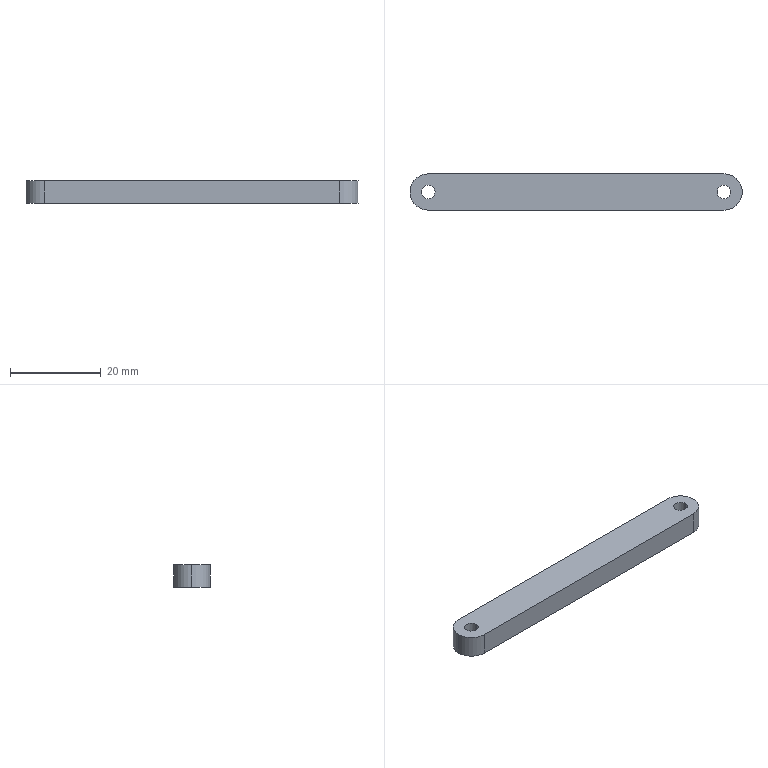Part | SolidWorks | features Extrusion 1, ICE 1 | 1 solid | 11 faces | box 73 x 8 x 5 mm | volume 2781 mm3 | cylinder 7 | plane 4 | commonest cylinder face diameters 3 x4 8 x3
STEP:
#1=CARTESIAN_POINT('',(-34.,0.,0.));
#2=VERTEX_POINT('',#1);
#3=CARTESIAN_POINT('',(-31.,0.,0.));
#4=VERTEX_POINT('',#3);
#5=CARTESIAN_POINT('',(-32.5,0.,0.));
#6=DIRECTION('',(0.,0.,1.));
#7=DIRECTION('',(1.,0.,0.));
#8=AXIS2_PLACEMENT_3D('',#5,#6,#7);
#9=CIRCLE('',#8,1.5);
#10=EDGE_CURVE('',#2,#4,#9,.T.);
#11=ORIENTED_EDGE('',*,*,#10,.F.);
#12=CARTESIAN_POINT('',(-34.,0.,5.));
#13=VERTEX_POINT('',#12);
#14=CARTESIAN_POINT('',(-34.,0.,0.));
#15=DIRECTION('',(0.,0.,1.));
#16=VECTOR('',#15,1000.);
#17=LINE('',#14,#16);
#18=EDGE_CURVE('',#2,#13,#17,.T.);
#19=ORIENTED_EDGE('',*,*,#18,.T.);
#20=CARTESIAN_POINT('',(-31.,0.,5.));
#21=VERTEX_POINT('',#20);
#22=CARTESIAN_POINT('',(-32.5,0.,5.));
#23=DIRECTION('',(0.,0.,1.));
#24=DIRECTION('',(1.,0.,0.));
#25=AXIS2_PLACEMENT_3D('',#22,#23,#24);
#26=CIRCLE('',#25,1.5);
#27=EDGE_CURVE('',#13,#21,#26,.T.);
#28=ORIENTED_EDGE('',*,*,#27,.T.);
#29=CARTESIAN_POINT('',(-31.,0.,0.));
#30=DIRECTION('',(0.,0.,1.));
#31=VECTOR('',#30,1000.);
#32=LINE('',#29,#31);
#33=EDGE_CURVE('',#4,#21,#32,.T.);
#34=ORIENTED_EDGE('',*,*,#33,.F.);
#35=EDGE_LOOP('',(#11,#19,#28,#34));
#36=FACE_OUTER_BOUND('',#35,.T.);
#37=CARTESIAN_POINT('',(-32.5,0.,0.));
#38=DIRECTION('',(0.,0.,1.));
#39=DIRECTION('',(1.,0.,0.));
#40=AXIS2_PLACEMENT_3D('',#37,#38,#39);
#41=CYLINDRICAL_SURFACE('',#40,1.5);
#42=ADVANCED_FACE('',(#36),#41,.F.);
#43=CARTESIAN_POINT('',(31.,0.,0.));
#44=VERTEX_POINT('',#43);
#45=CARTESIAN_POINT('',(34.,0.,0.));
#46=VERTEX_POINT('',#45);
#47=CARTESIAN_POINT('',(32.5,0.,0.));
#48=DIRECTION('',(0.,0.,1.));
#49=DIRECTION('',(1.,0.,0.));
#50=AXIS2_PLACEMENT_3D('',#47,#48,#49);
#51=CIRCLE('',#50,1.5);
#52=EDGE_CURVE('',#44,#46,#51,.T.);
#53=ORIENTED_EDGE('',*,*,#52,.F.);
#54=CARTESIAN_POINT('',(31.,0.,5.));
#55=VERTEX_POINT('',#54);
#56=CARTESIAN_POINT('',(31.,0.,0.));
#57=DIRECTION('',(0.,0.,1.));
#58=VECTOR('',#57,1000.);
#59=LINE('',#56,#58);
#60=EDGE_CURVE('',#44,#55,#59,.T.);
#61=ORIENTED_EDGE('',*,*,#60,.T.);
#62=CARTESIAN_POINT('',(34.,0.,5.));
#63=VERTEX_POINT('',#62);
#64=CARTESIAN_POINT('',(32.5,0.,5.));
#65=DIRECTION('',(0.,0.,1.));
#66=DIRECTION('',(1.,0.,0.));
#67=AXIS2_PLACEMENT_3D('',#64,#65,#66);
#68=CIRCLE('',#67,1.5);
#69=EDGE_CURVE('',#55,#63,#68,.T.);
#70=ORIENTED_EDGE('',*,*,#69,.T.);
#71=CARTESIAN_POINT('',(34.,0.,0.));
#72=DIRECTION('',(0.,0.,1.));
#73=VECTOR('',#72,1000.);
#74=LINE('',#71,#73);
#75=EDGE_CURVE('',#46,#63,#74,.T.);
#76=ORIENTED_EDGE('',*,*,#75,.F.);
#77=EDGE_LOOP('',(#53,#61,#70,#76));
#78=FACE_OUTER_BOUND('',#77,.T.);
#79=CARTESIAN_POINT('',(32.5,0.,0.));
#80=DIRECTION('',(0.,0.,1.));
#81=DIRECTION('',(1.,0.,0.));
#82=AXIS2_PLACEMENT_3D('',#79,#80,#81);
#83=CYLINDRICAL_SURFACE('',#82,1.5);
#84=ADVANCED_FACE('',(#78),#83,.F.);
#85=CARTESIAN_POINT('',(-36.5,0.,5.));
#86=VERTEX_POINT('',#85);
#87=CARTESIAN_POINT('',(-32.5,-4.,5.));
#88=VERTEX_POINT('',#87);
#89=CARTESIAN_POINT('',(-32.5,0.,5.));
#90=DIRECTION('',(0.,0.,1.));
#91=DIRECTION('',(1.,0.,0.));
#92=AXIS2_PLACEMENT_3D('',#89,#90,#91);
#93=CIRCLE('',#92,4.);
#94=EDGE_CURVE('',#86,#88,#93,.T.);
#95=ORIENTED_EDGE('',*,*,#94,.F.);
#96=CARTESIAN_POINT('',(-36.5,0.,0.));
#97=VERTEX_POINT('',#96);
#98=CARTESIAN_POINT('',(-36.5,0.,5.));
#99=DIRECTION('',(0.,0.,-1.));
#100=VECTOR('',#99,1000.);
#101=LINE('',#98,#100);
#102=EDGE_CURVE('',#86,#97,#101,.T.);
#103=ORIENTED_EDGE('',*,*,#102,.T.);
#104=CARTESIAN_POINT('',(-32.5,-4.,0.));
#105=VERTEX_POINT('',#104);
#106=CARTESIAN_POINT('',(-32.5,0.,0.));
#107=DIRECTION('',(0.,0.,1.));
#108=DIRECTION('',(1.,0.,0.));
#109=AXIS2_PLACEMENT_3D('',#106,#107,#108);
#110=CIRCLE('',#109,4.);
#111=EDGE_CURVE('',#97,#105,#110,.T.);
#112=ORIENTED_EDGE('',*,*,#111,.T.);
#113=CARTESIAN_POINT('',(-32.5,-4.,5.));
#114=DIRECTION('',(0.,0.,-1.));
#115=VECTOR('',#114,1000.);
#116=LINE('',#113,#115);
#117=EDGE_CURVE('',#88,#105,#116,.T.);
#118=ORIENTED_EDGE('',*,*,#117,.F.);
#119=EDGE_LOOP('',(#95,#103,#112,#118));
#120=FACE_OUTER_BOUND('',#119,.T.);
#121=CARTESIAN_POINT('',(-32.5,0.,5.));
#122=DIRECTION('',(0.,0.,-1.));
#123=DIRECTION('',(-1.,0.,0.));
#124=AXIS2_PLACEMENT_3D('',#121,#122,#123);
#125=CYLINDRICAL_SURFACE('',#124,4.);
#126=ADVANCED_FACE('',(#120),#125,.T.);
#127=ORIENTED_EDGE('',*,*,#102,.F.);
#128=CARTESIAN_POINT('',(-32.5,4.,5.));
#129=VERTEX_POINT('',#128);
#130=CARTESIAN_POINT('',(-32.5,0.,5.));
#131=DIRECTION('',(0.,0.,1.));
#132=DIRECTION('',(1.,0.,0.));
#133=AXIS2_PLACEMENT_3D('',#130,#131,#132);
#134=CIRCLE('',#133,4.);
#135=EDGE_CURVE('',#129,#86,#134,.T.);
#136=ORIENTED_EDGE('',*,*,#135,.F.);
#137=CARTESIAN_POINT('',(-32.5,4.,0.));
#138=VERTEX_POINT('',#137);
#139=CARTESIAN_POINT('',(-32.5,4.,5.));
#140=DIRECTION('',(0.,0.,-1.));
#141=VECTOR('',#140,1000.);
#142=LINE('',#139,#141);
#143=EDGE_CURVE('',#129,#138,#142,.T.);
#144=ORIENTED_EDGE('',*,*,#143,.T.);
#145=CARTESIAN_POINT('',(-32.5,0.,0.));
#146=DIRECTION('',(0.,0.,1.));
#147=DIRECTION('',(1.,0.,0.));
#148=AXIS2_PLACEMENT_3D('',#145,#146,#147);
#149=CIRCLE('',#148,4.);
#150=EDGE_CURVE('',#138,#97,#149,.T.);
#151=ORIENTED_EDGE('',*,*,#150,.T.);
#152=EDGE_LOOP('',(#127,#136,#144,#151));
#153=FACE_OUTER_BOUND('',#152,.T.);
#154=CARTESIAN_POINT('',(-32.5,0.,5.));
#155=DIRECTION('',(0.,0.,-1.));
#156=DIRECTION('',(-1.,0.,0.));
#157=AXIS2_PLACEMENT_3D('',#154,#155,#156);
#158=CYLINDRICAL_SURFACE('',#157,4.);
#159=ADVANCED_FACE('',(#153),#158,.T.);
#160=CARTESIAN_POINT('',(32.5,-4.,0.));
#161=VERTEX_POINT('',#160);
#162=CARTESIAN_POINT('',(-32.5,-4.,0.));
#163=DIRECTION('',(1.,0.,0.));
#164=VECTOR('',#163,1000.);
#165=LINE('',#162,#164);
#166=EDGE_CURVE('',#105,#161,#165,.T.);
#167=ORIENTED_EDGE('',*,*,#166,.T.);
#168=CARTESIAN_POINT('',(32.5,-4.,5.));
#169=VERTEX_POINT('',#168);
#170=CARTESIAN_POINT('',(32.5,-4.,5.));
#171=DIRECTION('',(0.,0.,-1.));
#172=VECTOR('',#171,1000.);
#173=LINE('',#170,#172);
#174=EDGE_CURVE('',#169,#161,#173,.T.);
#175=ORIENTED_EDGE('',*,*,#174,.F.);
#176=CARTESIAN_POINT('',(-32.5,-4.,5.));
#177=DIRECTION('',(1.,0.,0.));
#178=VECTOR('',#177,1000.);
#179=LINE('',#176,#178);
#180=EDGE_CURVE('',#88,#169,#179,.T.);
#181=ORIENTED_EDGE('',*,*,#180,.F.);
#182=ORIENTED_EDGE('',*,*,#117,.T.);
#183=EDGE_LOOP('',(#167,#175,#181,#182));
#184=FACE_OUTER_BOUND('',#183,.T.);
#185=CARTESIAN_POINT('',(-32.5,-4.,5.));
#186=DIRECTION('',(0.,1.,0.));
#187=DIRECTION('',(0.,0.,1.));
#188=AXIS2_PLACEMENT_3D('',#185,#186,#187);
#189=PLANE('',#188);
#190=ADVANCED_FACE('',(#184),#189,.F.);
#191=CARTESIAN_POINT('',(32.5,4.,0.));
#192=VERTEX_POINT('',#191);
#193=CARTESIAN_POINT('',(32.5,0.,0.));
#194=DIRECTION('',(0.,0.,1.));
#195=DIRECTION('',(1.,0.,0.));
#196=AXIS2_PLACEMENT_3D('',#193,#194,#195);
#197=CIRCLE('',#196,4.);
#198=EDGE_CURVE('',#161,#192,#197,.T.);
#199=ORIENTED_EDGE('',*,*,#198,.T.);
#200=CARTESIAN_POINT('',(32.5,4.,5.));
#201=VERTEX_POINT('',#200);
#202=CARTESIAN_POINT('',(32.5,4.,5.));
#203=DIRECTION('',(0.,0.,-1.));
#204=VECTOR('',#203,1000.);
#205=LINE('',#202,#204);
#206=EDGE_CURVE('',#201,#192,#205,.T.);
#207=ORIENTED_EDGE('',*,*,#206,.F.);
#208=CARTESIAN_POINT('',(32.5,0.,5.));
#209=DIRECTION('',(0.,0.,1.));
#210=DIRECTION('',(1.,0.,0.));
#211=AXIS2_PLACEMENT_3D('',#208,#209,#210);
#212=CIRCLE('',#211,4.);
#213=EDGE_CURVE('',#169,#201,#212,.T.);
#214=ORIENTED_EDGE('',*,*,#213,.F.);
#215=ORIENTED_EDGE('',*,*,#174,.T.);
#216=EDGE_LOOP('',(#199,#207,#214,#215));
#217=FACE_OUTER_BOUND('',#216,.T.);
#218=CARTESIAN_POINT('',(32.5,0.,5.));
#219=DIRECTION('',(0.,0.,-1.));
#220=DIRECTION('',(-1.,0.,0.));
#221=AXIS2_PLACEMENT_3D('',#218,#219,#220);
#222=CYLINDRICAL_SURFACE('',#221,4.);
#223=ADVANCED_FACE('',(#217),#222,.T.);
#224=CARTESIAN_POINT('',(-32.5,4.,0.));
#225=DIRECTION('',(-1.,0.,0.));
#226=VECTOR('',#225,1000.);
#227=LINE('',#224,#226);
#228=EDGE_CURVE('',#192,#138,#227,.T.);
#229=ORIENTED_EDGE('',*,*,#228,.T.);
#230=ORIENTED_EDGE('',*,*,#143,.F.);
#231=CARTESIAN_POINT('',(-32.5,4.,5.));
#232=DIRECTION('',(-1.,0.,0.));
#233=VECTOR('',#232,1000.);
#234=LINE('',#231,#233);
#235=EDGE_CURVE('',#201,#129,#234,.T.);
#236=ORIENTED_EDGE('',*,*,#235,.F.);
#237=ORIENTED_EDGE('',*,*,#206,.T.);
#238=EDGE_LOOP('',(#229,#230,#236,#237));
#239=FACE_OUTER_BOUND('',#238,.T.);
#240=CARTESIAN_POINT('',(-32.5,4.,5.));
#241=DIRECTION('',(0.,-1.,0.));
#242=DIRECTION('',(0.,0.,-1.));
#243=AXIS2_PLACEMENT_3D('',#240,#241,#242);
#244=PLANE('',#243);
#245=ADVANCED_FACE('',(#239),#244,.F.);
#246=CARTESIAN_POINT('',(-32.5,0.,5.));
#247=DIRECTION('',(0.,0.,1.));
#248=DIRECTION('',(1.,0.,0.));
#249=AXIS2_PLACEMENT_3D('',#246,#247,#248);
#250=CIRCLE('',#249,1.5);
#251=EDGE_CURVE('',#21,#13,#250,.T.);
#252=ORIENTED_EDGE('',*,*,#251,.F.);
#253=ORIENTED_EDGE('',*,*,#27,.F.);
#254=EDGE_LOOP('',(#252,#253));
#255=FACE_BOUND('',#254,.T.);
#256=CARTESIAN_POINT('',(32.5,0.,5.));
#257=DIRECTION('',(0.,0.,1.));
#258=DIRECTION('',(1.,0.,0.));
#259=AXIS2_PLACEMENT_3D('',#256,#257,#258);
#260=CIRCLE('',#259,1.5);
#261=EDGE_CURVE('',#63,#55,#260,.T.);
#262=ORIENTED_EDGE('',*,*,#261,.F.);
#263=ORIENTED_EDGE('',*,*,#69,.F.);
#264=EDGE_LOOP('',(#262,#263));
#265=FACE_BOUND('',#264,.T.);
#266=ORIENTED_EDGE('',*,*,#135,.T.);
#267=ORIENTED_EDGE('',*,*,#94,.T.);
#268=ORIENTED_EDGE('',*,*,#180,.T.);
#269=ORIENTED_EDGE('',*,*,#213,.T.);
#270=ORIENTED_EDGE('',*,*,#235,.T.);
#271=EDGE_LOOP('',(#266,#267,#268,#269,#270));
#272=FACE_OUTER_BOUND('',#271,.T.);
#273=CARTESIAN_POINT('',(-32.5,0.,5.));
#274=DIRECTION('',(0.,0.,1.));
#275=DIRECTION('',(1.,0.,0.));
#276=AXIS2_PLACEMENT_3D('',#273,#274,#275);
#277=PLANE('',#276);
#278=ADVANCED_FACE('',(#255,#265,#272),#277,.T.);
#279=CARTESIAN_POINT('',(-32.5,0.,0.));
#280=DIRECTION('',(0.,0.,1.));
#281=DIRECTION('',(1.,0.,0.));
#282=AXIS2_PLACEMENT_3D('',#279,#280,#281);
#283=CIRCLE('',#282,1.5);
#284=EDGE_CURVE('',#4,#2,#283,.T.);
#285=ORIENTED_EDGE('',*,*,#284,.T.);
#286=ORIENTED_EDGE('',*,*,#10,.T.);
#287=EDGE_LOOP('',(#285,#286));
#288=FACE_BOUND('',#287,.T.);
#289=CARTESIAN_POINT('',(32.5,0.,0.));
#290=DIRECTION('',(0.,0.,1.));
#291=DIRECTION('',(1.,0.,0.));
#292=AXIS2_PLACEMENT_3D('',#289,#290,#291);
#293=CIRCLE('',#292,1.5);
#294=EDGE_CURVE('',#46,#44,#293,.T.);
#295=ORIENTED_EDGE('',*,*,#294,.T.);
#296=ORIENTED_EDGE('',*,*,#52,.T.);
#297=EDGE_LOOP('',(#295,#296));
#298=FACE_BOUND('',#297,.T.);
#299=ORIENTED_EDGE('',*,*,#150,.F.);
#300=ORIENTED_EDGE('',*,*,#228,.F.);
#301=ORIENTED_EDGE('',*,*,#198,.F.);
#302=ORIENTED_EDGE('',*,*,#166,.F.);
#303=ORIENTED_EDGE('',*,*,#111,.F.);
#304=EDGE_LOOP('',(#299,#300,#301,#302,#303));
#305=FACE_OUTER_BOUND('',#304,.T.);
#306=CARTESIAN_POINT('',(-32.5,0.,0.));
#307=DIRECTION('',(0.,0.,1.));
#308=DIRECTION('',(1.,0.,0.));
#309=AXIS2_PLACEMENT_3D('',#306,#307,#308);
#310=PLANE('',#309);
#311=ADVANCED_FACE('',(#288,#298,#305),#310,.F.);
#312=ORIENTED_EDGE('',*,*,#60,.F.);
#313=ORIENTED_EDGE('',*,*,#294,.F.);
#314=ORIENTED_EDGE('',*,*,#75,.T.);
#315=ORIENTED_EDGE('',*,*,#261,.T.);
#316=EDGE_LOOP('',(#312,#313,#314,#315));
#317=FACE_OUTER_BOUND('',#316,.T.);
#318=CARTESIAN_POINT('',(32.5,0.,0.));
#319=DIRECTION('',(0.,0.,1.));
#320=DIRECTION('',(1.,0.,0.));
#321=AXIS2_PLACEMENT_3D('',#318,#319,#320);
#322=CYLINDRICAL_SURFACE('',#321,1.5);
#323=ADVANCED_FACE('',(#317),#322,.F.);
#324=ORIENTED_EDGE('',*,*,#18,.F.);
#325=ORIENTED_EDGE('',*,*,#284,.F.);
#326=ORIENTED_EDGE('',*,*,#33,.T.);
#327=ORIENTED_EDGE('',*,*,#251,.T.);
#328=EDGE_LOOP('',(#324,#325,#326,#327));
#329=FACE_OUTER_BOUND('',#328,.T.);
#330=CARTESIAN_POINT('',(-32.5,0.,0.));
#331=DIRECTION('',(0.,0.,1.));
#332=DIRECTION('',(1.,0.,0.));
#333=AXIS2_PLACEMENT_3D('',#330,#331,#332);
#334=CYLINDRICAL_SURFACE('',#333,1.5);
#335=ADVANCED_FACE('',(#329),#334,.F.);
#336=CLOSED_SHELL('',(#42,#84,#126,#159,#190,#223,#245,#278,#311,#323,#335));
#337=MANIFOLD_SOLID_BREP('',#336);
#338=CARTESIAN_POINT('',(0.,0.,0.));
#339=DIRECTION('',(0.,0.,1.));
#340=DIRECTION('',(1.,0.,0.));
#341=AXIS2_PLACEMENT_3D('',#338,#339,#340);
#342=(LENGTH_UNIT()NAMED_UNIT(*)SI_UNIT(.MILLI.,.METRE.));
#343=UNCERTAINTY_MEASURE_WITH_UNIT(LENGTH_MEASURE(0.00001),#342,'','');
#344=(NAMED_UNIT(*)PLANE_ANGLE_UNIT()SI_UNIT($,.RADIAN.));
#345=(NAMED_UNIT(*)SI_UNIT($,.STERADIAN.)SOLID_ANGLE_UNIT());
#346=(GEOMETRIC_REPRESENTATION_CONTEXT(3)GLOBAL_UNCERTAINTY_ASSIGNED_CONTEXT((#343))GLOBAL_UNIT_ASSIGNED_CONTEXT((#342,#344,#345))REPRESENTATION_CONTEXT('',''));
#347=ADVANCED_BREP_SHAPE_REPRESENTATION('',(#337,#341),#346);